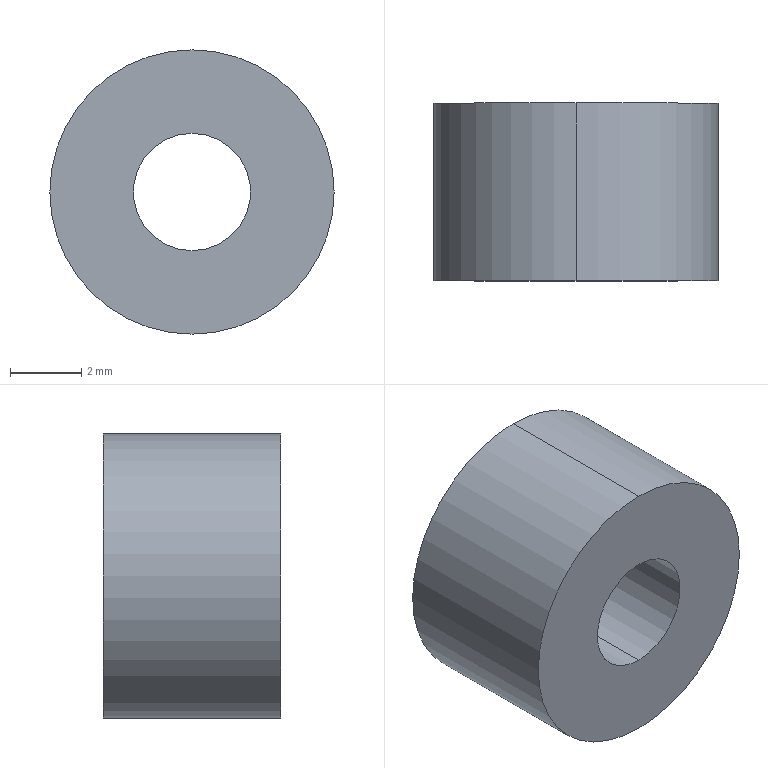Part | 1 solid | 6 faces | box 8 x 5 x 8 mm | volume 208.562 mm3 | cylinder 4 | plane 2 | commonest cylinder face diameters 3.3 x2 8 x2
STEP:
#1=CARTESIAN_POINT('',(0.,0.,-1.65));
#2=VERTEX_POINT('',#1);
#3=CARTESIAN_POINT('',(0.,0.,1.65));
#4=VERTEX_POINT('',#3);
#5=CARTESIAN_POINT('',(0.,0.,0.));
#6=DIRECTION('',(0.,1.,0.));
#7=DIRECTION('',(0.,0.,1.));
#8=AXIS2_PLACEMENT_3D('',#5,#6,#7);
#9=CIRCLE('',#8,1.65);
#10=EDGE_CURVE('',#2,#4,#9,.T.);
#11=ORIENTED_EDGE('',*,*,#10,.F.);
#12=CARTESIAN_POINT('',(0.,5.,-1.65));
#13=VERTEX_POINT('',#12);
#14=CARTESIAN_POINT('',(0.,5.,-1.65));
#15=DIRECTION('',(0.,1.,0.));
#16=VECTOR('',#15,1000.);
#17=LINE('',#14,#16);
#18=EDGE_CURVE('',#2,#13,#17,.T.);
#19=ORIENTED_EDGE('',*,*,#18,.T.);
#20=CARTESIAN_POINT('',(0.,5.,1.65));
#21=VERTEX_POINT('',#20);
#22=CARTESIAN_POINT('',(0.,5.,0.));
#23=DIRECTION('',(0.,1.,0.));
#24=DIRECTION('',(0.,0.,1.));
#25=AXIS2_PLACEMENT_3D('',#22,#23,#24);
#26=CIRCLE('',#25,1.65);
#27=EDGE_CURVE('',#13,#21,#26,.T.);
#28=ORIENTED_EDGE('',*,*,#27,.T.);
#29=CARTESIAN_POINT('',(0.,5.,1.65));
#30=DIRECTION('',(0.,1.,0.));
#31=VECTOR('',#30,1000.);
#32=LINE('',#29,#31);
#33=EDGE_CURVE('',#4,#21,#32,.T.);
#34=ORIENTED_EDGE('',*,*,#33,.F.);
#35=EDGE_LOOP('',(#11,#19,#28,#34));
#36=FACE_OUTER_BOUND('',#35,.T.);
#37=CARTESIAN_POINT('',(0.,5.,0.));
#38=DIRECTION('',(0.,1.,0.));
#39=DIRECTION('',(0.,0.,1.));
#40=AXIS2_PLACEMENT_3D('',#37,#38,#39);
#41=CYLINDRICAL_SURFACE('',#40,1.65);
#42=ADVANCED_FACE('',(#36),#41,.F.);
#43=CARTESIAN_POINT('',(0.,5.,4.));
#44=VERTEX_POINT('',#43);
#45=CARTESIAN_POINT('',(0.,5.,-4.));
#46=VERTEX_POINT('',#45);
#47=CARTESIAN_POINT('',(0.,5.,0.));
#48=DIRECTION('',(0.,1.,0.));
#49=DIRECTION('',(0.,0.,1.));
#50=AXIS2_PLACEMENT_3D('',#47,#48,#49);
#51=CIRCLE('',#50,4.);
#52=EDGE_CURVE('',#44,#46,#51,.T.);
#53=ORIENTED_EDGE('',*,*,#52,.F.);
#54=CARTESIAN_POINT('',(0.,0.,4.));
#55=VERTEX_POINT('',#54);
#56=CARTESIAN_POINT('',(0.,5.,4.));
#57=DIRECTION('',(0.,-1.,0.));
#58=VECTOR('',#57,1000.);
#59=LINE('',#56,#58);
#60=EDGE_CURVE('',#44,#55,#59,.T.);
#61=ORIENTED_EDGE('',*,*,#60,.T.);
#62=CARTESIAN_POINT('',(0.,0.,-4.));
#63=VERTEX_POINT('',#62);
#64=CARTESIAN_POINT('',(0.,0.,0.));
#65=DIRECTION('',(0.,1.,0.));
#66=DIRECTION('',(0.,0.,1.));
#67=AXIS2_PLACEMENT_3D('',#64,#65,#66);
#68=CIRCLE('',#67,4.);
#69=EDGE_CURVE('',#55,#63,#68,.T.);
#70=ORIENTED_EDGE('',*,*,#69,.T.);
#71=CARTESIAN_POINT('',(0.,5.,-4.));
#72=DIRECTION('',(0.,-1.,0.));
#73=VECTOR('',#72,1000.);
#74=LINE('',#71,#73);
#75=EDGE_CURVE('',#46,#63,#74,.T.);
#76=ORIENTED_EDGE('',*,*,#75,.F.);
#77=EDGE_LOOP('',(#53,#61,#70,#76));
#78=FACE_OUTER_BOUND('',#77,.T.);
#79=CARTESIAN_POINT('',(0.,5.,0.));
#80=DIRECTION('',(0.,-1.,0.));
#81=DIRECTION('',(0.,0.,-1.));
#82=AXIS2_PLACEMENT_3D('',#79,#80,#81);
#83=CYLINDRICAL_SURFACE('',#82,4.);
#84=ADVANCED_FACE('',(#78),#83,.T.);
#85=ORIENTED_EDGE('',*,*,#60,.F.);
#86=CARTESIAN_POINT('',(0.,5.,0.));
#87=DIRECTION('',(0.,1.,0.));
#88=DIRECTION('',(0.,0.,1.));
#89=AXIS2_PLACEMENT_3D('',#86,#87,#88);
#90=CIRCLE('',#89,4.);
#91=EDGE_CURVE('',#46,#44,#90,.T.);
#92=ORIENTED_EDGE('',*,*,#91,.F.);
#93=ORIENTED_EDGE('',*,*,#75,.T.);
#94=CARTESIAN_POINT('',(0.,0.,0.));
#95=DIRECTION('',(0.,1.,0.));
#96=DIRECTION('',(0.,0.,1.));
#97=AXIS2_PLACEMENT_3D('',#94,#95,#96);
#98=CIRCLE('',#97,4.);
#99=EDGE_CURVE('',#63,#55,#98,.T.);
#100=ORIENTED_EDGE('',*,*,#99,.T.);
#101=EDGE_LOOP('',(#85,#92,#93,#100));
#102=FACE_OUTER_BOUND('',#101,.T.);
#103=CARTESIAN_POINT('',(0.,5.,0.));
#104=DIRECTION('',(0.,-1.,0.));
#105=DIRECTION('',(0.,0.,-1.));
#106=AXIS2_PLACEMENT_3D('',#103,#104,#105);
#107=CYLINDRICAL_SURFACE('',#106,4.);
#108=ADVANCED_FACE('',(#102),#107,.T.);
#109=CARTESIAN_POINT('',(0.,5.,0.));
#110=DIRECTION('',(0.,1.,0.));
#111=DIRECTION('',(0.,0.,1.));
#112=AXIS2_PLACEMENT_3D('',#109,#110,#111);
#113=CIRCLE('',#112,1.65);
#114=EDGE_CURVE('',#21,#13,#113,.T.);
#115=ORIENTED_EDGE('',*,*,#114,.F.);
#116=ORIENTED_EDGE('',*,*,#27,.F.);
#117=EDGE_LOOP('',(#115,#116));
#118=FACE_BOUND('',#117,.T.);
#119=ORIENTED_EDGE('',*,*,#91,.T.);
#120=ORIENTED_EDGE('',*,*,#52,.T.);
#121=EDGE_LOOP('',(#119,#120));
#122=FACE_OUTER_BOUND('',#121,.T.);
#123=CARTESIAN_POINT('',(0.,5.,0.));
#124=DIRECTION('',(0.,1.,0.));
#125=DIRECTION('',(0.,0.,1.));
#126=AXIS2_PLACEMENT_3D('',#123,#124,#125);
#127=PLANE('',#126);
#128=ADVANCED_FACE('',(#118,#122),#127,.T.);
#129=CARTESIAN_POINT('',(0.,0.,0.));
#130=DIRECTION('',(0.,1.,0.));
#131=DIRECTION('',(0.,0.,1.));
#132=AXIS2_PLACEMENT_3D('',#129,#130,#131);
#133=CIRCLE('',#132,1.65);
#134=EDGE_CURVE('',#4,#2,#133,.T.);
#135=ORIENTED_EDGE('',*,*,#134,.T.);
#136=ORIENTED_EDGE('',*,*,#10,.T.);
#137=EDGE_LOOP('',(#135,#136));
#138=FACE_BOUND('',#137,.T.);
#139=ORIENTED_EDGE('',*,*,#99,.F.);
#140=ORIENTED_EDGE('',*,*,#69,.F.);
#141=EDGE_LOOP('',(#139,#140));
#142=FACE_OUTER_BOUND('',#141,.T.);
#143=CARTESIAN_POINT('',(0.,0.,0.));
#144=DIRECTION('',(0.,1.,0.));
#145=DIRECTION('',(0.,0.,1.));
#146=AXIS2_PLACEMENT_3D('',#143,#144,#145);
#147=PLANE('',#146);
#148=ADVANCED_FACE('',(#138,#142),#147,.F.);
#149=ORIENTED_EDGE('',*,*,#18,.F.);
#150=ORIENTED_EDGE('',*,*,#134,.F.);
#151=ORIENTED_EDGE('',*,*,#33,.T.);
#152=ORIENTED_EDGE('',*,*,#114,.T.);
#153=EDGE_LOOP('',(#149,#150,#151,#152));
#154=FACE_OUTER_BOUND('',#153,.T.);
#155=CARTESIAN_POINT('',(0.,5.,0.));
#156=DIRECTION('',(0.,1.,0.));
#157=DIRECTION('',(0.,0.,1.));
#158=AXIS2_PLACEMENT_3D('',#155,#156,#157);
#159=CYLINDRICAL_SURFACE('',#158,1.65);
#160=ADVANCED_FACE('',(#154),#159,.F.);
#161=CLOSED_SHELL('',(#42,#84,#108,#128,#148,#160));
#162=MANIFOLD_SOLID_BREP('',#161);
#163=CARTESIAN_POINT('',(0.,0.,0.));
#164=DIRECTION('',(0.,0.,1.));
#165=DIRECTION('',(1.,0.,0.));
#166=AXIS2_PLACEMENT_3D('',#163,#164,#165);
#167=(LENGTH_UNIT()NAMED_UNIT(*)SI_UNIT(.MILLI.,.METRE.));
#168=UNCERTAINTY_MEASURE_WITH_UNIT(LENGTH_MEASURE(0.00001),#167,'','');
#169=(NAMED_UNIT(*)PLANE_ANGLE_UNIT()SI_UNIT($,.RADIAN.));
#170=(NAMED_UNIT(*)SI_UNIT($,.STERADIAN.)SOLID_ANGLE_UNIT());
#171=(GEOMETRIC_REPRESENTATION_CONTEXT(3)GLOBAL_UNCERTAINTY_ASSIGNED_CONTEXT((#168))GLOBAL_UNIT_ASSIGNED_CONTEXT((#167,#169,#170))REPRESENTATION_CONTEXT('',''));
#172=ADVANCED_BREP_SHAPE_REPRESENTATION('',(#162,#166),#171);